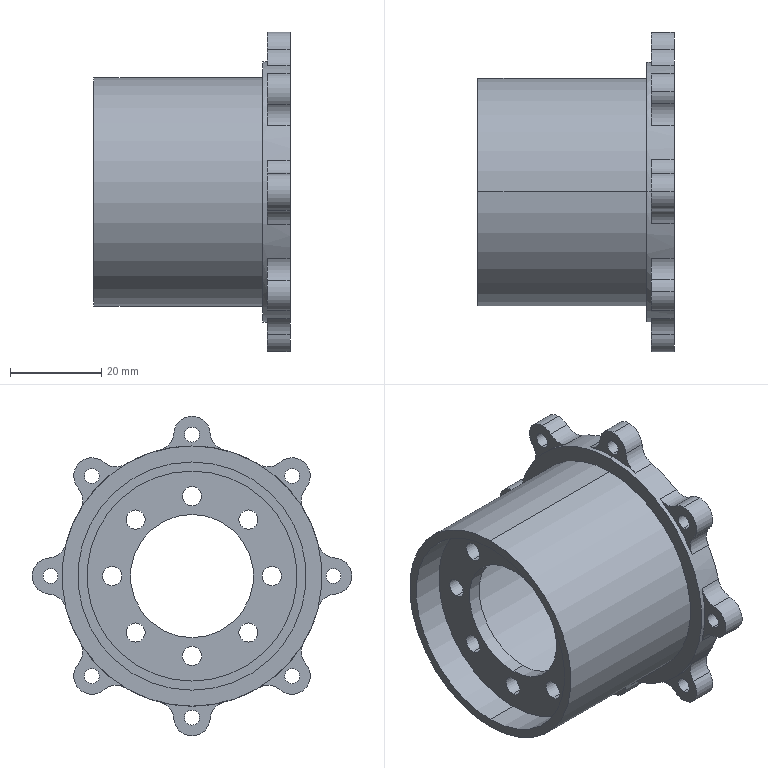Part | SolidWorks | features ICE 4, HoleWzd 1, Revolution 1 | 1 solid | 100 faces | box 43 x 70 x 70 mm | volume 21080 mm3 | cylinder 71 | cone 16 | plane 13 | commonest cylinder face diameters 8 x29 3.3 x16 4.2 x16 46 x4 27 x2 50 x2